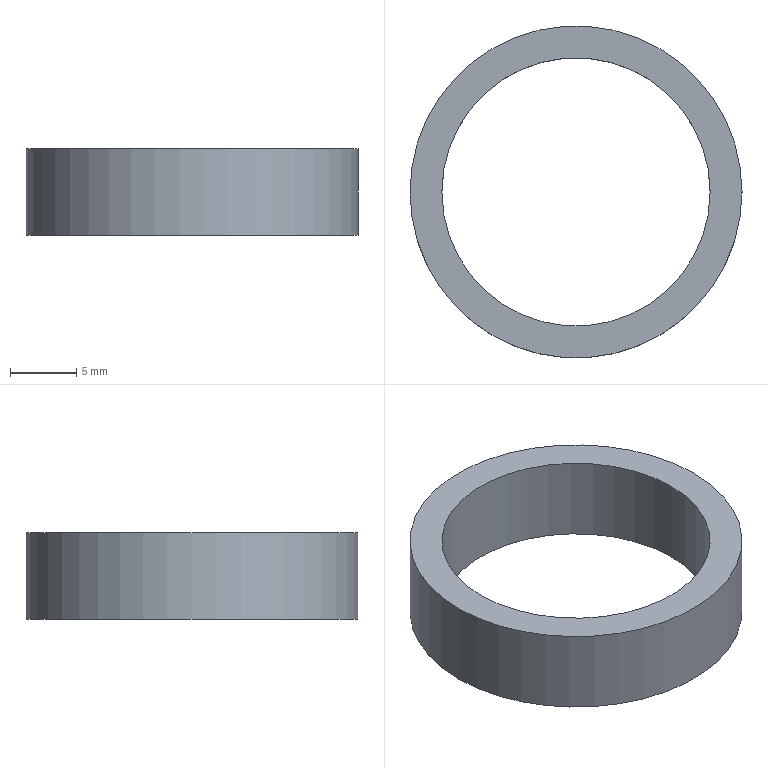Part | NX | features DATUM_CSYS 1, EXTRACT_DATUM_PLANE 1, EXTRUDE 1, SKETCH 1 | 1 solid | 4 faces | box 25 x 25 x 6.5 mm | volume 1108 mm3 | cylinder 2 | plane 2 | commonest cylinder face diameters 20.2 x1 25 x1
STEP:
#1=CARTESIAN_POINT('',(-12.5,0.,0.));
#2=VERTEX_POINT('',#1);
#3=CARTESIAN_POINT('',(0.,0.,0.));
#4=DIRECTION('',(0.,0.,-1.));
#5=DIRECTION('',(-1.,0.,0.));
#6=AXIS2_PLACEMENT_3D('',#3,#4,#5);
#7=CIRCLE('',#6,12.5);
#8=EDGE_CURVE('',#2,#2,#7,.T.);
#9=ORIENTED_EDGE('',*,*,#8,.F.);
#10=EDGE_LOOP('',(#9));
#11=FACE_BOUND('',#10,.T.);
#12=CARTESIAN_POINT('',(12.5,0.,6.5));
#13=VERTEX_POINT('',#12);
#14=CARTESIAN_POINT('',(0.,0.,6.5));
#15=DIRECTION('',(0.,0.,-1.));
#16=DIRECTION('',(1.,0.,0.));
#17=AXIS2_PLACEMENT_3D('',#14,#15,#16);
#18=CIRCLE('',#17,12.5);
#19=EDGE_CURVE('',#13,#13,#18,.T.);
#20=ORIENTED_EDGE('',*,*,#19,.T.);
#21=EDGE_LOOP('',(#20));
#22=FACE_BOUND('',#21,.T.);
#23=CARTESIAN_POINT('',(0.,0.,6.5));
#24=DIRECTION('',(0.,0.,-1.));
#25=DIRECTION('',(-1.,0.,0.));
#26=AXIS2_PLACEMENT_3D('',#23,#24,#25);
#27=CYLINDRICAL_SURFACE('',#26,12.5);
#28=ADVANCED_FACE('',(#11,#22),#27,.T.);
#29=CARTESIAN_POINT('',(-10.1,0.,0.));
#30=VERTEX_POINT('',#29);
#31=CARTESIAN_POINT('',(0.,0.,0.));
#32=DIRECTION('',(0.,0.,-1.));
#33=DIRECTION('',(-1.,0.,0.));
#34=AXIS2_PLACEMENT_3D('',#31,#32,#33);
#35=CIRCLE('',#34,10.1);
#36=EDGE_CURVE('',#30,#30,#35,.T.);
#37=ORIENTED_EDGE('',*,*,#36,.T.);
#38=EDGE_LOOP('',(#37));
#39=FACE_BOUND('',#38,.T.);
#40=CARTESIAN_POINT('',(10.1,0.,6.5));
#41=VERTEX_POINT('',#40);
#42=CARTESIAN_POINT('',(0.,0.,6.5));
#43=DIRECTION('',(0.,0.,-1.));
#44=DIRECTION('',(1.,0.,0.));
#45=AXIS2_PLACEMENT_3D('',#42,#43,#44);
#46=CIRCLE('',#45,10.1);
#47=EDGE_CURVE('',#41,#41,#46,.T.);
#48=ORIENTED_EDGE('',*,*,#47,.F.);
#49=EDGE_LOOP('',(#48));
#50=FACE_BOUND('',#49,.T.);
#51=CARTESIAN_POINT('',(0.,0.,6.5));
#52=DIRECTION('',(0.,0.,-1.));
#53=DIRECTION('',(-1.,0.,0.));
#54=AXIS2_PLACEMENT_3D('',#51,#52,#53);
#55=CYLINDRICAL_SURFACE('',#54,10.1);
#56=ADVANCED_FACE('',(#39,#50),#55,.F.);
#57=ORIENTED_EDGE('',*,*,#19,.F.);
#58=EDGE_LOOP('',(#57));
#59=FACE_BOUND('',#58,.T.);
#60=ORIENTED_EDGE('',*,*,#47,.T.);
#61=EDGE_LOOP('',(#60));
#62=FACE_BOUND('',#61,.T.);
#63=CARTESIAN_POINT('',(0.,0.,6.5));
#64=DIRECTION('',(0.,0.,-1.));
#65=DIRECTION('',(-1.,0.,0.));
#66=AXIS2_PLACEMENT_3D('',#63,#64,#65);
#67=PLANE('',#66);
#68=ADVANCED_FACE('',(#59,#62),#67,.F.);
#69=ORIENTED_EDGE('',*,*,#8,.T.);
#70=EDGE_LOOP('',(#69));
#71=FACE_BOUND('',#70,.T.);
#72=ORIENTED_EDGE('',*,*,#36,.F.);
#73=EDGE_LOOP('',(#72));
#74=FACE_BOUND('',#73,.T.);
#75=CARTESIAN_POINT('',(0.,0.,0.));
#76=DIRECTION('',(0.,0.,-1.));
#77=DIRECTION('',(-1.,0.,0.));
#78=AXIS2_PLACEMENT_3D('',#75,#76,#77);
#79=PLANE('',#78);
#80=ADVANCED_FACE('',(#71,#74),#79,.T.);
#81=CLOSED_SHELL('',(#28,#56,#68,#80));
#82=MANIFOLD_SOLID_BREP('',#81);
#83=(LENGTH_UNIT()NAMED_UNIT(*)SI_UNIT(.MILLI.,.METRE.));
#84=UNCERTAINTY_MEASURE_WITH_UNIT(LENGTH_MEASURE(0.00001),#83,'','');
#85=(NAMED_UNIT(*)PLANE_ANGLE_UNIT()SI_UNIT($,.RADIAN.));
#86=(NAMED_UNIT(*)SI_UNIT($,.STERADIAN.)SOLID_ANGLE_UNIT());
#87=(GEOMETRIC_REPRESENTATION_CONTEXT(3)GLOBAL_UNCERTAINTY_ASSIGNED_CONTEXT((#84))GLOBAL_UNIT_ASSIGNED_CONTEXT((#83,#85,#86))REPRESENTATION_CONTEXT('',''));
#88=ADVANCED_BREP_SHAPE_REPRESENTATION('',(#82),#87);